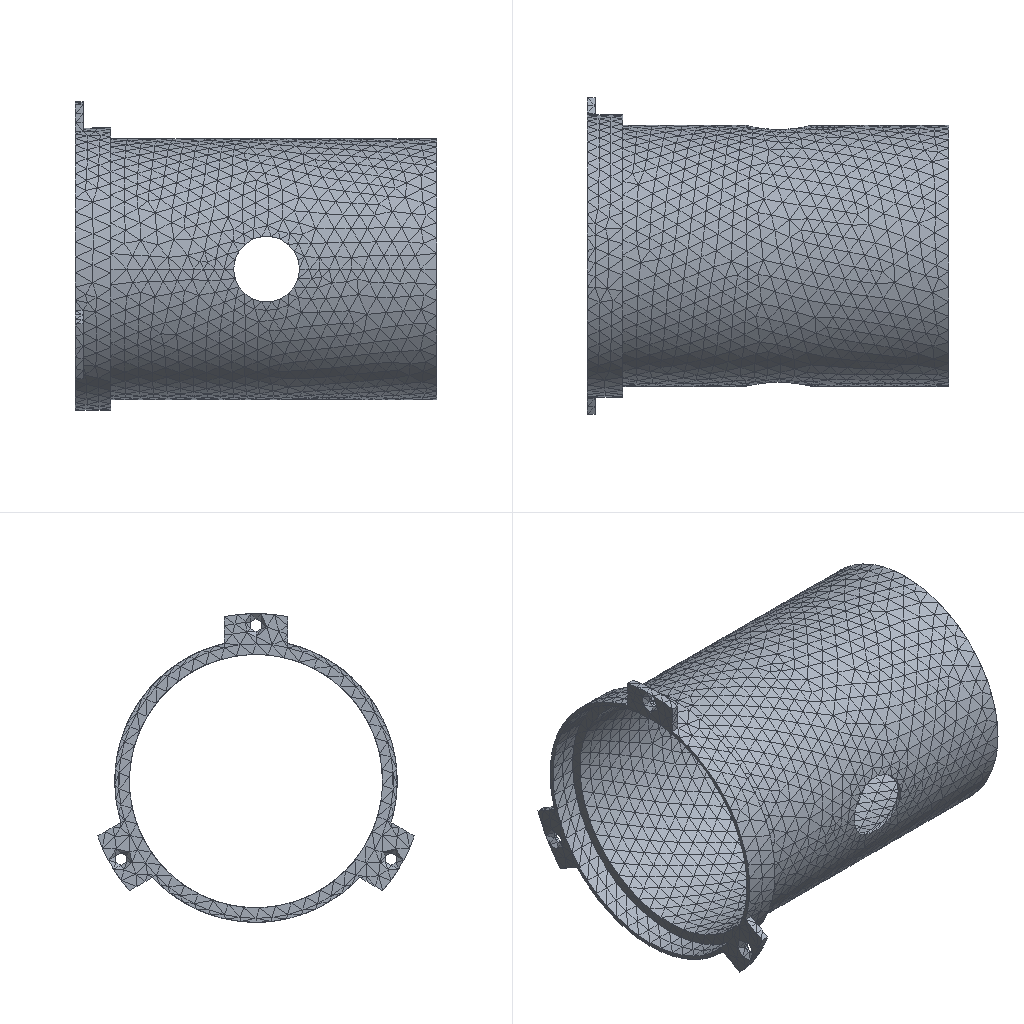Simulation study | nx simcenter
Set-up summary:
category,name,step,type,value,unit,region
solver,nx_nastran (Simcenter)
units,not stated in the deck,,not stated
analysis,deck,,static,static
analysis,solution,,SOL,101
load_step,SUBCASE 1,1,SUBCASE,SPC=1 LOAD=2
load_step,requested,,,1
mesh,nodes,,,18365
mesh,elements,,,8903
element_type,CTETRA,,solid,8903
load,nodal force total,,FX,-3499999.98,model units
load,nodal force total,,FY,0.0,model units
load,nodal force total,,FZ,0.0,model units
load,load commands in deck,,count,204
bc,support commands in deck,,count,489
analysis,NX solution 0,,Structural,Linear Statics - Single Constraint
check,setup vs results,,match,every grid point's frame and coordinates and every element id; grid points of CTETRA elements
Nastran input file, long lists of numbers shortened:
$*$$$$$$$$$$$$$$$$$$$$$$$$$$$$$$$$$$$$$$$$$$$$$$$$$$$$$$$$$$$$$$$$$
$*
$*                    NX v10.0.0.24 TRANSLATOR
$*                    FOR NX NASTRAN VERSION 10.0
$ (33 more lines like these left out)
ASSIGN OUTPUT2='160_sim1-solution_1.op2' UNIT=12
$*
$*$$$$$$$$$$$$$$$$$$$$$$$$$$$$$$$$$$$
$*
$* EXECUTIVE CONTROL
$*
$*$$$$$$$$$$$$$$$$$$$$$$$$$$$$$$$$$$$
$*
ID,NASTRAN,160_sim1-solution_1
SOL 101
CEND
$*
$*$$$$$$$$$$$$$$$$$$$$$$$$$$$$$$$$$$$
$*
$* CASE CONTROL
$*
$*$$$$$$$$$$$$$$$$$$$$$$$$$$$$$$$$$$$
$*
TITLE = Solution 1
ECHO = NONE
SPC = 1
OUTPUT
BCRESULTS(TRACTION,FORCE,PLOT) = ALL
DISPLACEMENT(PLOT) = ALL
ESE(PLOT) = ALL
FORCE(PLOT,CORNER) = ALL
OLOAD(PLOT) = ALL
SPCFORCES(PLOT) = ALL
STRAIN(PLOT,FIBER,CORNER) = ALL
STRESS(PLOT,CORNER) = ALL
$*  NX Step: Subcase - Static Loads 1
SUBCASE 1
LABEL = Subcase - Static Loads 1
LOAD = 2
$*
$*$$$$$$$$$$$$$$$$$$$$$$$$$$$$$$$$$$$
$*
$* BULK DATA
$*
$*$$$$$$$$$$$$$$$$$$$$$$$$$$$$$$$$$$$
$*
BEGIN BULK
$*
$* PARAM CARDS
$*
PARAM      K6ROT100.0000
PARAM     OIBULK     YES
PARAM    OMACHPR     YES
PARAM       POST      -2
PARAM    POSTEXT     YES
PARAM    UNITSYS   MN-MM
$*
$* GRID CARDS
$*
GRID*              18311               0-1.500000000E+00-5.115182877E+01+
*       -1.567611504E+01               0
GRID*              18312               0-1.500000000E+00-6.000173569E+01+
*       -2.078561020E+01               0
$ (36726 more lines like these left out)
$*
$* ELEMENT CARDS
$*
$*  NX Mesh Collector: Solid(1)
$*  NX Mesh: 3d_mesh(1)
CTETRA         1       1    7593    7456   12820    7588    9947       1+
+              2    9939    9946       3
CTETRA         2       1    7457   12806   12807   12813       4   15860+
+              5       6   15859   15844
$ (17802 more lines like these left out)
$*
$* PROPERTY CARDS
$*
$*  NX Property: PSOLID1
PSOLID         1       1       0                           SMECH
$*
$* MATERIAL CARDS
$*
$*  NX Material: 7075
MAT1           12.0000+8        0.3300002.8100-62.1355-5
MATT1          1                       1               2
TABLEM1        1                                                        +
+        20.00000.330000 21.11000.330000    ENDT
TABLEM1        2                                                        +
+        20.00002.1600-5 93.33002.2500-5107.22002.2662-5121.11002.2824-5+
+       135.00002.2968-5148.89002.3130-5162.78002.3274-5176.67002.3418-5+
+       190.56002.3544-5204.44002.3688-5218.33002.3814-5232.22002.3958-5+
+       246.11002.4066-5260.00002.4192-5273.89002.4300-5287.78002.4408-5+
+       301.67002.4498-5315.56002.4606-5329.44002.4696-5343.33002.4786-5+
+       357.22002.4876-5371.11002.4984-5385.00002.5110-5398.89002.5254-5+
+       412.78002.5398-5426.67002.5560-5    ENDT
$*
$* LOAD AND CONSTRAINT CARDS
$*
$*  NX Load and Constraint: Fixed(1)
SPC            1   16761  123456  0.0000
SPC            1   16762  123456  0.0000
SPC            1   16763  123456  0.0000
SPC            1   16764  123456  0.0000
$ (485 more lines like these left out)
$*  NX Load and Constraint: Force(1)
FORCE          2   16659       022883.59-1.00000  0.0000  0.0000
FORCE          2   16660       022814.82-1.00000  0.0000  0.0000
FORCE          2   16661       022807.66-1.00000  0.0000  0.0000
FORCE          2   16662       022881.93-1.00000  0.0000  0.0000
$ (200 more lines like these left out)
ENDDATA b04f76d0
Results summary:
result,analysis,,,static
result,last_loadstep,,,1
result,primary field,,,displacements
result,max displacement,,,0.01209,model units
result,reaction total,,FX,3499999.0,model units
result,reaction total,,FY,0.2061,model units
result,reaction total,,FZ,0.1533,model units
result,NX solution 0,,loadcases,1,mm